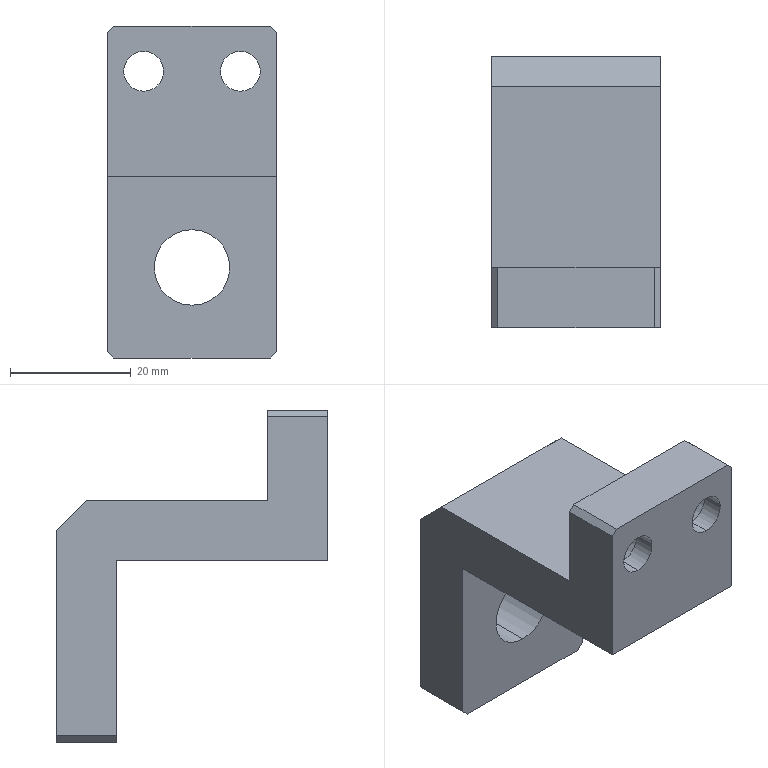Part | STEP file | PN_0030 | 1 solid | 27 faces | box 28 x 45 x 55 mm | volume 22140 mm3 | plane 17 | cylinder 10 | commonest cylinder face diameters 6.6 x4 11 x4 12.5 x2